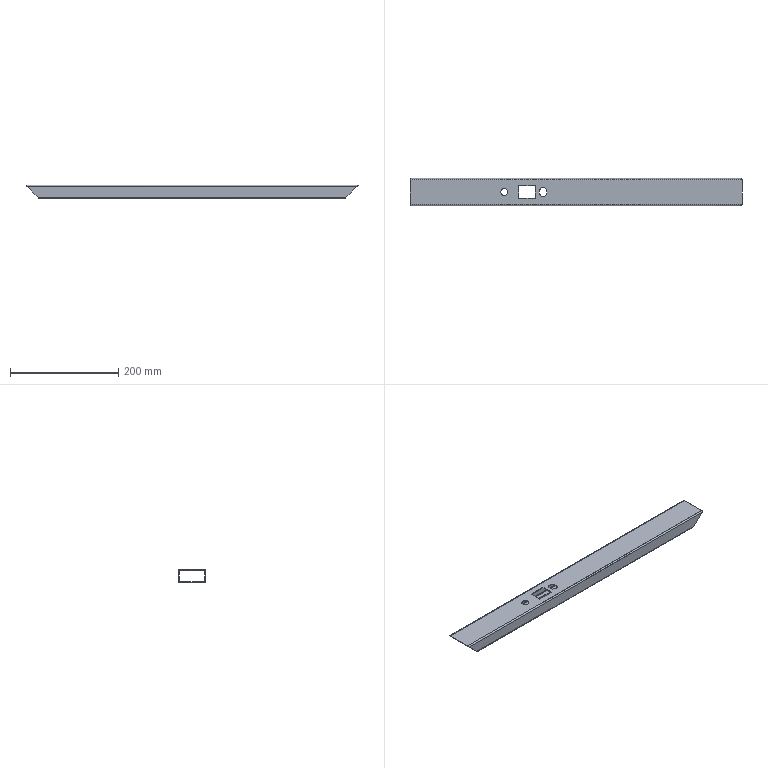Part | STEP file | 6100502 | 1 solid | 31 faces | box 613 x 50 x 25 mm | volume 116984 mm3 | plane 20 | cylinder 11 | commonest cylinder face diameters 2 x4 5 x4 15.8 x2 13 x1